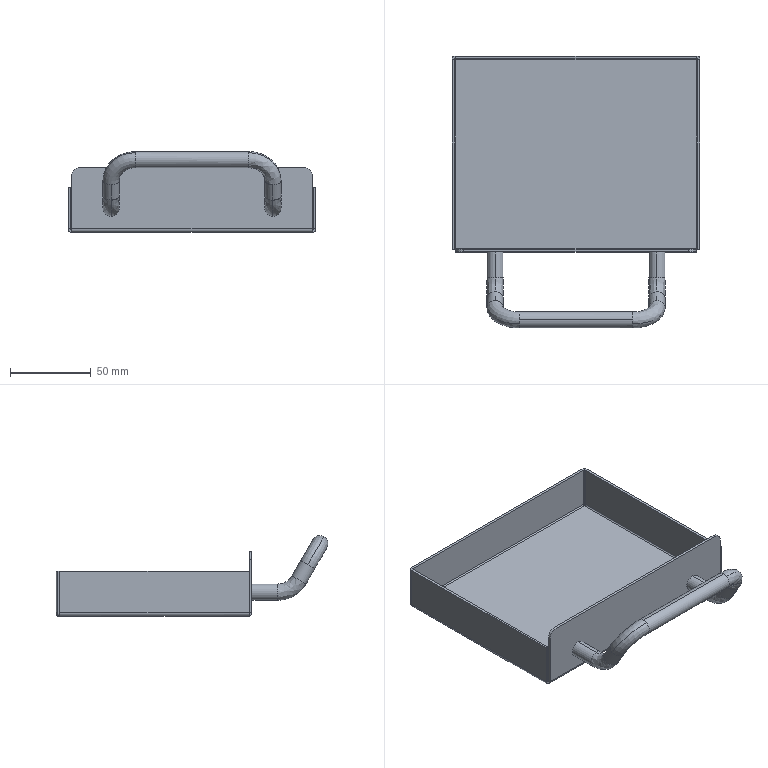Part | STEP file | 03-25 scrap box (Default) | 2 solids | 101 faces | box 153 x 168 x 50 mm | volume 66699 mm3 | plane 45 | cylinder 30 | spline 18 | cone 8 | commonest cylinder face diameters 10 x8 1.473 x4 4.134 x4 4.473 x4 4.5 x4 9.998 x4